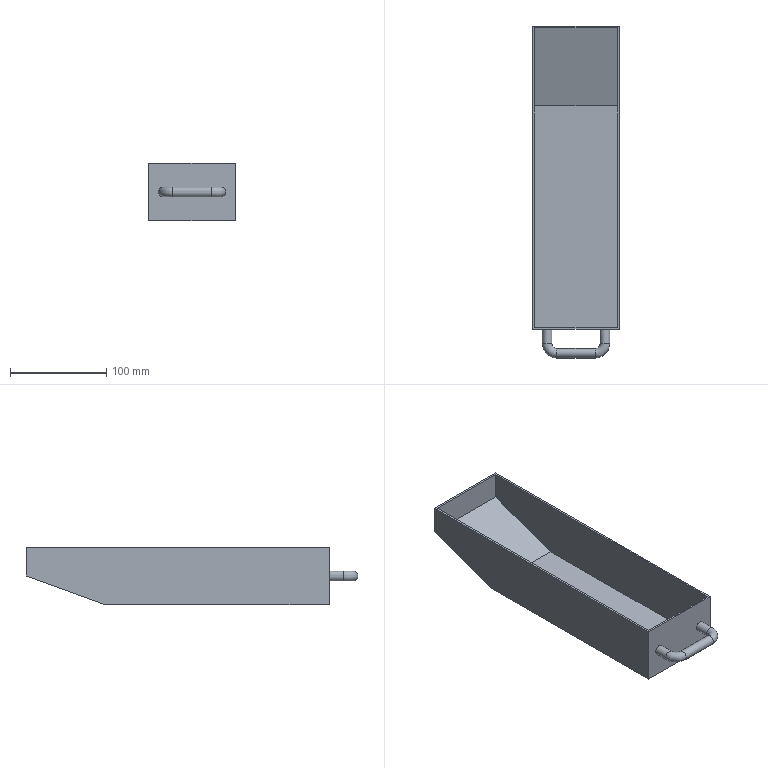Part | NX | features solid 2 | 1 solid | 18 faces | box 90 x 345 x 60 mm | volume 148544 mm3 | plane 13 | cylinder 3 | torus 2 | commonest cylinder face diameters 10 x3
STEP:
#1=CARTESIAN_POINT('',(-180.,35.,-255.));
#2=VERTEX_POINT('',#1);
#3=CARTESIAN_POINT('',(-180.,-47.424,-285.));
#4=VERTEX_POINT('',#3);
#5=CARTESIAN_POINT('',(-180.,18.93,-260.849));
#6=DIRECTION('',(0.,-0.9397,-0.342));
#7=VECTOR('',#6,1000.);
#8=LINE('',#5,#7);
#9=EDGE_CURVE('',#2,#4,#8,.T.);
#10=ORIENTED_EDGE('',*,*,#9,.F.);
#11=CARTESIAN_POINT('',(-180.,35.,-225.));
#12=VERTEX_POINT('',#11);
#13=CARTESIAN_POINT('',(-180.,35.,-305.));
#14=DIRECTION('',(0.,0.,1.));
#15=VECTOR('',#14,1000.);
#16=LINE('',#13,#15);
#17=EDGE_CURVE('',#2,#12,#16,.T.);
#18=ORIENTED_EDGE('',*,*,#17,.T.);
#19=CARTESIAN_POINT('',(-180.,-280.,-225.));
#20=VERTEX_POINT('',#19);
#21=CARTESIAN_POINT('',(-180.,35.,-225.));
#22=DIRECTION('',(0.,-1.,0.));
#23=VECTOR('',#22,1000.);
#24=LINE('',#21,#23);
#25=EDGE_CURVE('',#12,#20,#24,.T.);
#26=ORIENTED_EDGE('',*,*,#25,.T.);
#27=CARTESIAN_POINT('',(-180.,-280.,-285.));
#28=VERTEX_POINT('',#27);
#29=CARTESIAN_POINT('',(-180.,-280.,-145.));
#30=DIRECTION('',(0.,0.,-1.));
#31=VECTOR('',#30,1000.);
#32=LINE('',#29,#31);
#33=EDGE_CURVE('',#28,#20,#32,.F.);
#34=ORIENTED_EDGE('',*,*,#33,.F.);
#35=CARTESIAN_POINT('',(-180.,35.,-285.));
#36=DIRECTION('',(0.,-1.,0.));
#37=VECTOR('',#36,1000.);
#38=LINE('',#35,#37);
#39=EDGE_CURVE('',#4,#28,#38,.T.);
#40=ORIENTED_EDGE('',*,*,#39,.F.);
#41=EDGE_LOOP('',(#10,#18,#26,#34,#40));
#42=FACE_BOUND('',#41,.T.);
#43=CARTESIAN_POINT('',(-180.,35.,-305.));
#44=DIRECTION('',(-1.,0.,0.));
#45=DIRECTION('',(0.,0.,1.));
#46=AXIS2_PLACEMENT_3D('',#43,#44,#45);
#47=PLANE('',#46);
#48=ADVANCED_FACE('',(#42),#47,.F.);
#49=CARTESIAN_POINT('',(-270.,-47.424,-285.));
#50=VERTEX_POINT('',#49);
#51=CARTESIAN_POINT('',(-270.,35.,-255.));
#52=VERTEX_POINT('',#51);
#53=CARTESIAN_POINT('',(-270.,-268.052,-365.302));
#54=DIRECTION('',(0.,0.9397,0.342));
#55=VECTOR('',#54,1000.);
#56=LINE('',#53,#55);
#57=EDGE_CURVE('',#50,#52,#56,.T.);
#58=ORIENTED_EDGE('',*,*,#57,.F.);
#59=CARTESIAN_POINT('',(-270.,-280.,-285.));
#60=VERTEX_POINT('',#59);
#61=CARTESIAN_POINT('',(-270.,-290.,-285.));
#62=DIRECTION('',(0.,1.,0.));
#63=VECTOR('',#62,1000.);
#64=LINE('',#61,#63);
#65=EDGE_CURVE('',#60,#50,#64,.T.);
#66=ORIENTED_EDGE('',*,*,#65,.F.);
#67=CARTESIAN_POINT('',(-270.,-280.,-225.));
#68=VERTEX_POINT('',#67);
#69=CARTESIAN_POINT('',(-270.,-280.,-305.));
#70=DIRECTION('',(0.,0.,-1.));
#71=VECTOR('',#70,1000.);
#72=LINE('',#69,#71);
#73=EDGE_CURVE('',#60,#68,#72,.F.);
#74=ORIENTED_EDGE('',*,*,#73,.T.);
#75=CARTESIAN_POINT('',(-270.,35.,-225.));
#76=VERTEX_POINT('',#75);
#77=CARTESIAN_POINT('',(-270.,-290.,-225.));
#78=DIRECTION('',(0.,1.,0.));
#79=VECTOR('',#78,1000.);
#80=LINE('',#77,#79);
#81=EDGE_CURVE('',#68,#76,#80,.T.);
#82=ORIENTED_EDGE('',*,*,#81,.T.);
#83=CARTESIAN_POINT('',(-270.,35.,-305.));
#84=DIRECTION('',(0.,0.,1.));
#85=VECTOR('',#84,1000.);
#86=LINE('',#83,#85);
#87=EDGE_CURVE('',#52,#76,#86,.T.);
#88=ORIENTED_EDGE('',*,*,#87,.F.);
#89=EDGE_LOOP('',(#58,#66,#74,#82,#88));
#90=FACE_BOUND('',#89,.T.);
#91=CARTESIAN_POINT('',(-270.,-290.,-305.));
#92=DIRECTION('',(1.,0.,0.));
#93=DIRECTION('',(0.,0.,-1.));
#94=AXIS2_PLACEMENT_3D('',#91,#92,#93);
#95=PLANE('',#94);
#96=ADVANCED_FACE('',(#90),#95,.F.);
#97=CARTESIAN_POINT('',(-270.,35.,-255.));
#98=DIRECTION('',(1.,0.,0.));
#99=VECTOR('',#98,1000.);
#100=LINE('',#97,#99);
#101=EDGE_CURVE('',#52,#2,#100,.T.);
#102=ORIENTED_EDGE('',*,*,#101,.F.);
#103=ORIENTED_EDGE('',*,*,#87,.T.);
#104=CARTESIAN_POINT('',(-270.,35.,-225.));
#105=DIRECTION('',(1.,0.,0.));
#106=VECTOR('',#105,1000.);
#107=LINE('',#104,#106);
#108=EDGE_CURVE('',#76,#12,#107,.T.);
#109=ORIENTED_EDGE('',*,*,#108,.T.);
#110=ORIENTED_EDGE('',*,*,#17,.F.);
#111=EDGE_LOOP('',(#102,#103,#109,#110));
#112=FACE_BOUND('',#111,.T.);
#113=CARTESIAN_POINT('',(-270.,35.,-305.));
#114=DIRECTION('',(0.,-1.,0.));
#115=DIRECTION('',(0.,0.,-1.));
#116=AXIS2_PLACEMENT_3D('',#113,#114,#115);
#117=PLANE('',#116);
#118=ADVANCED_FACE('',(#112),#117,.F.);
#119=ORIENTED_EDGE('',*,*,#65,.T.);
#120=CARTESIAN_POINT('',(-180.,-47.424,-285.));
#121=DIRECTION('',(1.,0.,0.));
#122=VECTOR('',#121,1000.);
#123=LINE('',#120,#122);
#124=EDGE_CURVE('',#50,#4,#123,.T.);
#125=ORIENTED_EDGE('',*,*,#124,.T.);
#126=ORIENTED_EDGE('',*,*,#39,.T.);
#127=CARTESIAN_POINT('',(-690.,-280.,-285.));
#128=DIRECTION('',(1.,0.,0.));
#129=VECTOR('',#128,1000.);
#130=LINE('',#127,#129);
#131=EDGE_CURVE('',#28,#60,#130,.F.);
#132=ORIENTED_EDGE('',*,*,#131,.T.);
#133=EDGE_LOOP('',(#119,#125,#126,#132));
#134=FACE_BOUND('',#133,.T.);
#135=CARTESIAN_POINT('',(-180.,-290.,-285.));
#136=DIRECTION('',(0.,0.,-1.));
#137=DIRECTION('',(-1.,0.,0.));
#138=AXIS2_PLACEMENT_3D('',#135,#136,#137);
#139=PLANE('',#138);
#140=ADVANCED_FACE('',(#134),#139,.T.);
#141=CARTESIAN_POINT('',(-182.,-47.777,-283.));
#142=VERTEX_POINT('',#141);
#143=CARTESIAN_POINT('',(-182.,33.,-253.6));
#144=VERTEX_POINT('',#143);
#145=CARTESIAN_POINT('',(-182.,18.246,-258.97));
#146=DIRECTION('',(0.,0.9397,0.342));
#147=VECTOR('',#146,1000.);
#148=LINE('',#145,#147);
#149=EDGE_CURVE('',#142,#144,#148,.T.);
#150=ORIENTED_EDGE('',*,*,#149,.F.);
#151=CARTESIAN_POINT('',(-182.,-278.,-283.));
#152=VERTEX_POINT('',#151);
#153=CARTESIAN_POINT('',(-182.,35.,-283.));
#154=DIRECTION('',(0.,-1.,0.));
#155=VECTOR('',#154,1000.);
#156=LINE('',#153,#155);
#157=EDGE_CURVE('',#142,#152,#156,.T.);
#158=ORIENTED_EDGE('',*,*,#157,.T.);
#159=CARTESIAN_POINT('',(-182.,-278.,-225.));
#160=VERTEX_POINT('',#159);
#161=CARTESIAN_POINT('',(-182.,-278.,-145.));
#162=DIRECTION('',(0.,0.,-1.));
#163=VECTOR('',#162,1000.);
#164=LINE('',#161,#163);
#165=EDGE_CURVE('',#152,#160,#164,.F.);
#166=ORIENTED_EDGE('',*,*,#165,.T.);
#167=CARTESIAN_POINT('',(-182.,33.,-225.));
#168=VERTEX_POINT('',#167);
#169=CARTESIAN_POINT('',(-182.,35.,-225.));
#170=DIRECTION('',(0.,-1.,0.));
#171=VECTOR('',#170,1000.);
#172=LINE('',#169,#171);
#173=EDGE_CURVE('',#168,#160,#172,.T.);
#174=ORIENTED_EDGE('',*,*,#173,.F.);
#175=CARTESIAN_POINT('',(-182.,33.,-305.));
#176=DIRECTION('',(0.,0.,1.));
#177=VECTOR('',#176,1000.);
#178=LINE('',#175,#177);
#179=EDGE_CURVE('',#144,#168,#178,.T.);
#180=ORIENTED_EDGE('',*,*,#179,.F.);
#181=EDGE_LOOP('',(#150,#158,#166,#174,#180));
#182=FACE_BOUND('',#181,.T.);
#183=CARTESIAN_POINT('',(-182.,35.,-305.));
#184=DIRECTION('',(-1.,0.,0.));
#185=DIRECTION('',(0.,0.,1.));
#186=AXIS2_PLACEMENT_3D('',#183,#184,#185);
#187=PLANE('',#186);
#188=ADVANCED_FACE('',(#182),#187,.T.);
#189=CARTESIAN_POINT('',(-268.,33.,-253.6));
#190=VERTEX_POINT('',#189);
#191=CARTESIAN_POINT('',(-268.,-47.777,-283.));
#192=VERTEX_POINT('',#191);
#193=CARTESIAN_POINT('',(-268.,-268.736,-363.422));
#194=DIRECTION('',(0.,-0.9397,-0.342));
#195=VECTOR('',#194,1000.);
#196=LINE('',#193,#195);
#197=EDGE_CURVE('',#190,#192,#196,.T.);
#198=ORIENTED_EDGE('',*,*,#197,.F.);
#199=CARTESIAN_POINT('',(-268.,33.,-225.));
#200=VERTEX_POINT('',#199);
#201=CARTESIAN_POINT('',(-268.,33.,-305.));
#202=DIRECTION('',(0.,0.,1.));
#203=VECTOR('',#202,1000.);
#204=LINE('',#201,#203);
#205=EDGE_CURVE('',#190,#200,#204,.T.);
#206=ORIENTED_EDGE('',*,*,#205,.T.);
#207=CARTESIAN_POINT('',(-268.,-278.,-225.));
#208=VERTEX_POINT('',#207);
#209=CARTESIAN_POINT('',(-268.,-290.,-225.));
#210=DIRECTION('',(0.,1.,0.));
#211=VECTOR('',#210,1000.);
#212=LINE('',#209,#211);
#213=EDGE_CURVE('',#208,#200,#212,.T.);
#214=ORIENTED_EDGE('',*,*,#213,.F.);
#215=CARTESIAN_POINT('',(-268.,-278.,-283.));
#216=VERTEX_POINT('',#215);
#217=CARTESIAN_POINT('',(-268.,-278.,-305.));
#218=DIRECTION('',(0.,0.,-1.));
#219=VECTOR('',#218,1000.);
#220=LINE('',#217,#219);
#221=EDGE_CURVE('',#216,#208,#220,.F.);
#222=ORIENTED_EDGE('',*,*,#221,.F.);
#223=CARTESIAN_POINT('',(-268.,-290.,-283.));
#224=DIRECTION('',(0.,1.,0.));
#225=VECTOR('',#224,1000.);
#226=LINE('',#223,#225);
#227=EDGE_CURVE('',#216,#192,#226,.T.);
#228=ORIENTED_EDGE('',*,*,#227,.T.);
#229=EDGE_LOOP('',(#198,#206,#214,#222,#228));
#230=FACE_BOUND('',#229,.T.);
#231=CARTESIAN_POINT('',(-268.,-290.,-305.));
#232=DIRECTION('',(1.,0.,0.));
#233=DIRECTION('',(0.,0.,-1.));
#234=AXIS2_PLACEMENT_3D('',#231,#232,#233);
#235=PLANE('',#234);
#236=ADVANCED_FACE('',(#230),#235,.T.);
#237=CARTESIAN_POINT('',(-270.,33.,-253.6));
#238=DIRECTION('',(-1.,0.,0.));
#239=VECTOR('',#238,1000.);
#240=LINE('',#237,#239);
#241=EDGE_CURVE('',#144,#190,#240,.T.);
#242=ORIENTED_EDGE('',*,*,#241,.F.);
#243=ORIENTED_EDGE('',*,*,#179,.T.);
#244=CARTESIAN_POINT('',(-270.,33.,-225.));
#245=DIRECTION('',(1.,0.,0.));
#246=VECTOR('',#245,1000.);
#247=LINE('',#244,#246);
#248=EDGE_CURVE('',#200,#168,#247,.T.);
#249=ORIENTED_EDGE('',*,*,#248,.F.);
#250=ORIENTED_EDGE('',*,*,#205,.F.);
#251=EDGE_LOOP('',(#242,#243,#249,#250));
#252=FACE_BOUND('',#251,.T.);
#253=CARTESIAN_POINT('',(-270.,33.,-305.));
#254=DIRECTION('',(0.,-1.,0.));
#255=DIRECTION('',(0.,0.,-1.));
#256=AXIS2_PLACEMENT_3D('',#253,#254,#255);
#257=PLANE('',#256);
#258=ADVANCED_FACE('',(#252),#257,.T.);
#259=ORIENTED_EDGE('',*,*,#157,.F.);
#260=CARTESIAN_POINT('',(-180.,-47.777,-283.));
#261=DIRECTION('',(-1.,0.,0.));
#262=VECTOR('',#261,1000.);
#263=LINE('',#260,#262);
#264=EDGE_CURVE('',#142,#192,#263,.T.);
#265=ORIENTED_EDGE('',*,*,#264,.T.);
#266=ORIENTED_EDGE('',*,*,#227,.F.);
#267=CARTESIAN_POINT('',(-690.,-278.,-283.));
#268=DIRECTION('',(1.,0.,0.));
#269=VECTOR('',#268,1000.);
#270=LINE('',#267,#269);
#271=EDGE_CURVE('',#152,#216,#270,.F.);
#272=ORIENTED_EDGE('',*,*,#271,.F.);
#273=EDGE_LOOP('',(#259,#265,#266,#272));
#274=FACE_BOUND('',#273,.T.);
#275=CARTESIAN_POINT('',(-180.,-290.,-283.));
#276=DIRECTION('',(0.,0.,-1.));
#277=DIRECTION('',(-1.,0.,0.));
#278=AXIS2_PLACEMENT_3D('',#275,#276,#277);
#279=PLANE('',#278);
#280=ADVANCED_FACE('',(#274),#279,.F.);
#281=CARTESIAN_POINT('',(-255.,-280.,-260.));
#282=VERTEX_POINT('',#281);
#283=CARTESIAN_POINT('',(-255.,-280.,-255.));
#284=DIRECTION('',(0.,1.,0.));
#285=DIRECTION('',(0.,0.,-1.));
#286=AXIS2_PLACEMENT_3D('',#283,#284,#285);
#287=CIRCLE('',#286,5.);
#288=EDGE_CURVE('',#282,#282,#287,.T.);
#289=ORIENTED_EDGE('',*,*,#288,.T.);
#290=EDGE_LOOP('',(#289));
#291=FACE_BOUND('',#290,.T.);
#292=CARTESIAN_POINT('',(-690.,-280.,-225.));
#293=DIRECTION('',(1.,0.,0.));
#294=VECTOR('',#293,1000.);
#295=LINE('',#292,#294);
#296=EDGE_CURVE('',#20,#68,#295,.F.);
#297=ORIENTED_EDGE('',*,*,#296,.T.);
#298=ORIENTED_EDGE('',*,*,#73,.F.);
#299=ORIENTED_EDGE('',*,*,#131,.F.);
#300=ORIENTED_EDGE('',*,*,#33,.T.);
#301=EDGE_LOOP('',(#297,#298,#299,#300));
#302=FACE_BOUND('',#301,.T.);
#303=CARTESIAN_POINT('',(-190.,-280.,-255.));
#304=VERTEX_POINT('',#303);
#305=CARTESIAN_POINT('',(-195.,-280.,-255.));
#306=DIRECTION('',(0.,-1.,0.));
#307=DIRECTION('',(1.,0.,0.));
#308=AXIS2_PLACEMENT_3D('',#305,#306,#307);
#309=CIRCLE('',#308,5.);
#310=EDGE_CURVE('',#304,#304,#309,.T.);
#311=ORIENTED_EDGE('',*,*,#310,.F.);
#312=EDGE_LOOP('',(#311));
#313=FACE_BOUND('',#312,.T.);
#314=CARTESIAN_POINT('',(-690.,-280.,-145.));
#315=DIRECTION('',(0.,-1.,0.));
#316=DIRECTION('',(1.,0.,0.));
#317=AXIS2_PLACEMENT_3D('',#314,#315,#316);
#318=PLANE('',#317);
#319=ADVANCED_FACE('',(#291,#302,#313),#318,.T.);
#320=ORIENTED_EDGE('',*,*,#248,.T.);
#321=ORIENTED_EDGE('',*,*,#173,.T.);
#322=CARTESIAN_POINT('',(-690.,-278.,-225.));
#323=DIRECTION('',(1.,0.,0.));
#324=VECTOR('',#323,1000.);
#325=LINE('',#322,#324);
#326=EDGE_CURVE('',#160,#208,#325,.F.);
#327=ORIENTED_EDGE('',*,*,#326,.T.);
#328=ORIENTED_EDGE('',*,*,#213,.T.);
#329=EDGE_LOOP('',(#320,#321,#327,#328));
#330=FACE_BOUND('',#329,.T.);
#331=ORIENTED_EDGE('',*,*,#25,.F.);
#332=ORIENTED_EDGE('',*,*,#108,.F.);
#333=ORIENTED_EDGE('',*,*,#81,.F.);
#334=ORIENTED_EDGE('',*,*,#296,.F.);
#335=EDGE_LOOP('',(#331,#332,#333,#334));
#336=FACE_BOUND('',#335,.T.);
#337=CARTESIAN_POINT('',(-180.,-290.,-225.));
#338=DIRECTION('',(0.,0.,-1.));
#339=DIRECTION('',(-1.,0.,0.));
#340=AXIS2_PLACEMENT_3D('',#337,#338,#339);
#341=PLANE('',#340);
#342=ADVANCED_FACE('',(#330,#336),#341,.F.);
#343=ORIENTED_EDGE('',*,*,#326,.F.);
#344=ORIENTED_EDGE('',*,*,#165,.F.);
#345=ORIENTED_EDGE('',*,*,#271,.T.);
#346=ORIENTED_EDGE('',*,*,#221,.T.);
#347=EDGE_LOOP('',(#343,#344,#345,#346));
#348=FACE_BOUND('',#347,.T.);
#349=CARTESIAN_POINT('',(-690.,-278.,-145.));
#350=DIRECTION('',(0.,-1.,0.));
#351=DIRECTION('',(1.,0.,0.));
#352=AXIS2_PLACEMENT_3D('',#349,#350,#351);
#353=PLANE('',#352);
#354=ADVANCED_FACE('',(#348),#353,.F.);
#355=CARTESIAN_POINT('',(-255.,-295.,-260.));
#356=VERTEX_POINT('',#355);
#357=CARTESIAN_POINT('',(-255.,-295.,-255.));
#358=DIRECTION('',(0.,1.,0.));
#359=DIRECTION('',(0.,0.,-1.));
#360=AXIS2_PLACEMENT_3D('',#357,#358,#359);
#361=CIRCLE('',#360,5.);
#362=EDGE_CURVE('',#356,#356,#361,.T.);
#363=ORIENTED_EDGE('',*,*,#362,.T.);
#364=EDGE_LOOP('',(#363));
#365=FACE_BOUND('',#364,.T.);
#366=ORIENTED_EDGE('',*,*,#288,.F.);
#367=EDGE_LOOP('',(#366));
#368=FACE_BOUND('',#367,.T.);
#369=CARTESIAN_POINT('',(-255.,-295.,-255.));
#370=DIRECTION('',(0.,1.,0.));
#371=DIRECTION('',(0.,0.,1.));
#372=AXIS2_PLACEMENT_3D('',#369,#370,#371);
#373=CYLINDRICAL_SURFACE('',#372,5.);
#374=ADVANCED_FACE('',(#365,#368),#373,.T.);
#375=CARTESIAN_POINT('',(-245.,-305.,-260.));
#376=VERTEX_POINT('',#375);
#377=CARTESIAN_POINT('',(-245.,-305.,-255.));
#378=DIRECTION('',(-1.,0.,0.));
#379=DIRECTION('',(0.,0.,-1.));
#380=AXIS2_PLACEMENT_3D('',#377,#378,#379);
#381=CIRCLE('',#380,5.);
#382=EDGE_CURVE('',#376,#376,#381,.T.);
#383=ORIENTED_EDGE('',*,*,#382,.T.);
#384=EDGE_LOOP('',(#383));
#385=FACE_BOUND('',#384,.T.);
#386=ORIENTED_EDGE('',*,*,#362,.F.);
#387=EDGE_LOOP('',(#386));
#388=FACE_BOUND('',#387,.T.);
#389=CARTESIAN_POINT('',(-245.,-295.,-255.));
#390=DIRECTION('',(0.,0.,-1.));
#391=DIRECTION('',(-1.,0.,0.));
#392=AXIS2_PLACEMENT_3D('',#389,#390,#391);
#393=TOROIDAL_SURFACE('',#392,10.,5.);
#394=ADVANCED_FACE('',(#385,#388),#393,.T.);
#395=CARTESIAN_POINT('',(-205.,-305.,-260.));
#396=VERTEX_POINT('',#395);
#397=CARTESIAN_POINT('',(-205.,-305.,-255.));
#398=DIRECTION('',(-1.,0.,0.));
#399=DIRECTION('',(0.,0.,-1.));
#400=AXIS2_PLACEMENT_3D('',#397,#398,#399);
#401=CIRCLE('',#400,5.);
#402=EDGE_CURVE('',#396,#396,#401,.T.);
#403=ORIENTED_EDGE('',*,*,#402,.T.);
#404=EDGE_LOOP('',(#403));
#405=FACE_BOUND('',#404,.T.);
#406=ORIENTED_EDGE('',*,*,#382,.F.);
#407=EDGE_LOOP('',(#406));
#408=FACE_BOUND('',#407,.T.);
#409=CARTESIAN_POINT('',(-205.,-305.,-255.));
#410=DIRECTION('',(-1.,0.,0.));
#411=DIRECTION('',(0.,0.,1.));
#412=AXIS2_PLACEMENT_3D('',#409,#410,#411);
#413=CYLINDRICAL_SURFACE('',#412,5.);
#414=ADVANCED_FACE('',(#405,#408),#413,.T.);
#415=CARTESIAN_POINT('',(-195.,-295.,-260.));
#416=VERTEX_POINT('',#415);
#417=CARTESIAN_POINT('',(-195.,-295.,-255.));
#418=DIRECTION('',(0.,-1.,0.));
#419=DIRECTION('',(0.,0.,-1.));
#420=AXIS2_PLACEMENT_3D('',#417,#418,#419);
#421=CIRCLE('',#420,5.);
#422=EDGE_CURVE('',#416,#416,#421,.T.);
#423=ORIENTED_EDGE('',*,*,#422,.T.);
#424=EDGE_LOOP('',(#423));
#425=FACE_BOUND('',#424,.T.);
#426=ORIENTED_EDGE('',*,*,#402,.F.);
#427=EDGE_LOOP('',(#426));
#428=FACE_BOUND('',#427,.T.);
#429=CARTESIAN_POINT('',(-205.,-295.,-255.));
#430=DIRECTION('',(0.,0.,-1.));
#431=DIRECTION('',(-1.,0.,0.));
#432=AXIS2_PLACEMENT_3D('',#429,#430,#431);
#433=TOROIDAL_SURFACE('',#432,10.,5.);
#434=ADVANCED_FACE('',(#425,#428),#433,.T.);
#435=ORIENTED_EDGE('',*,*,#422,.F.);
#436=EDGE_LOOP('',(#435));
#437=FACE_BOUND('',#436,.T.);
#438=ORIENTED_EDGE('',*,*,#310,.T.);
#439=EDGE_LOOP('',(#438));
#440=FACE_BOUND('',#439,.T.);
#441=CARTESIAN_POINT('',(-195.,-295.,-255.));
#442=DIRECTION('',(0.,1.,0.));
#443=DIRECTION('',(0.,0.,1.));
#444=AXIS2_PLACEMENT_3D('',#441,#442,#443);
#445=CYLINDRICAL_SURFACE('',#444,5.);
#446=ADVANCED_FACE('',(#437,#440),#445,.T.);
#447=ORIENTED_EDGE('',*,*,#57,.T.);
#448=ORIENTED_EDGE('',*,*,#101,.T.);
#449=ORIENTED_EDGE('',*,*,#9,.T.);
#450=ORIENTED_EDGE('',*,*,#124,.F.);
#451=EDGE_LOOP('',(#447,#448,#449,#450));
#452=FACE_BOUND('',#451,.T.);
#453=CARTESIAN_POINT('',(-180.,-261.003,-362.736));
#454=DIRECTION('',(0.,0.342,-0.9397));
#455=DIRECTION('',(0.,0.9397,0.342));
#456=AXIS2_PLACEMENT_3D('',#453,#454,#455);
#457=PLANE('',#456);
#458=ADVANCED_FACE('',(#452),#457,.T.);
#459=ORIENTED_EDGE('',*,*,#149,.T.);
#460=ORIENTED_EDGE('',*,*,#241,.T.);
#461=ORIENTED_EDGE('',*,*,#197,.T.);
#462=ORIENTED_EDGE('',*,*,#264,.F.);
#463=EDGE_LOOP('',(#459,#460,#461,#462));
#464=FACE_BOUND('',#463,.T.);
#465=CARTESIAN_POINT('',(-230.,34.316,-253.121));
#466=DIRECTION('',(0.,-0.342,0.9397));
#467=DIRECTION('',(0.,-0.9397,-0.342));
#468=AXIS2_PLACEMENT_3D('',#465,#466,#467);
#469=PLANE('',#468);
#470=ADVANCED_FACE('',(#464),#469,.T.);
#471=CLOSED_SHELL('',(#48,#96,#118,#140,#188,#236,#258,#280,#319,#342,#354,#374,#394,#414,#434,#446,#458,#470));
#472=MANIFOLD_SOLID_BREP('',#471);
#473=(LENGTH_UNIT()NAMED_UNIT(*)SI_UNIT(.MILLI.,.METRE.));
#474=UNCERTAINTY_MEASURE_WITH_UNIT(LENGTH_MEASURE(0.00001),#473,'','');
#475=(NAMED_UNIT(*)PLANE_ANGLE_UNIT()SI_UNIT($,.RADIAN.));
#476=(NAMED_UNIT(*)SI_UNIT($,.STERADIAN.)SOLID_ANGLE_UNIT());
#477=(GEOMETRIC_REPRESENTATION_CONTEXT(3)GLOBAL_UNCERTAINTY_ASSIGNED_CONTEXT((#474))GLOBAL_UNIT_ASSIGNED_CONTEXT((#473,#475,#476))REPRESENTATION_CONTEXT('',''));
#478=ADVANCED_BREP_SHAPE_REPRESENTATION('',(#472),#477);